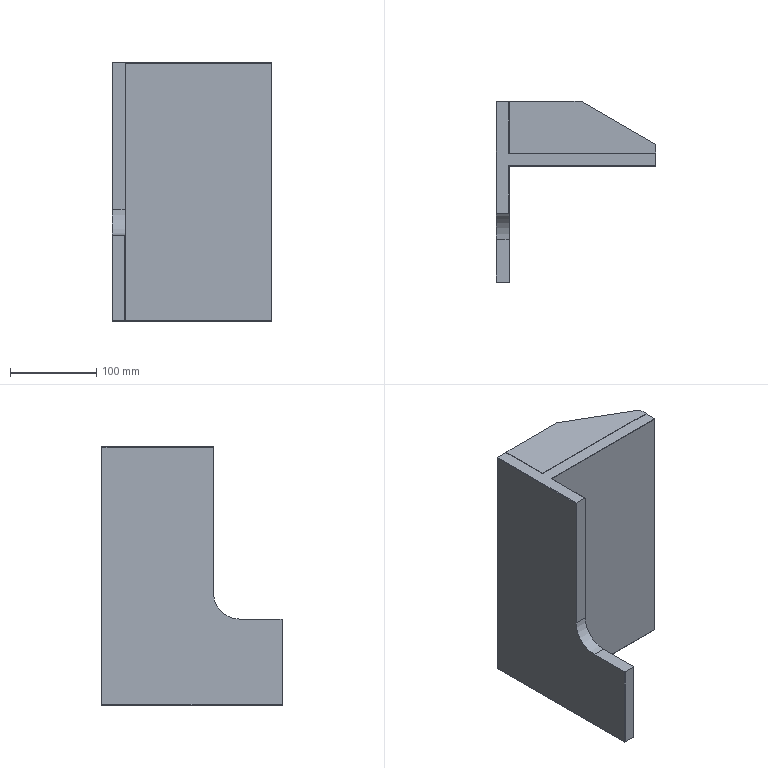Part | STEP file | HJDX-202 | 4 solids | 65 faces | box 185 x 210 x 300 mm | volume 1834119 mm3 | plane 64 | cylinder 1 | commonest cylinder face diameters 60 x1